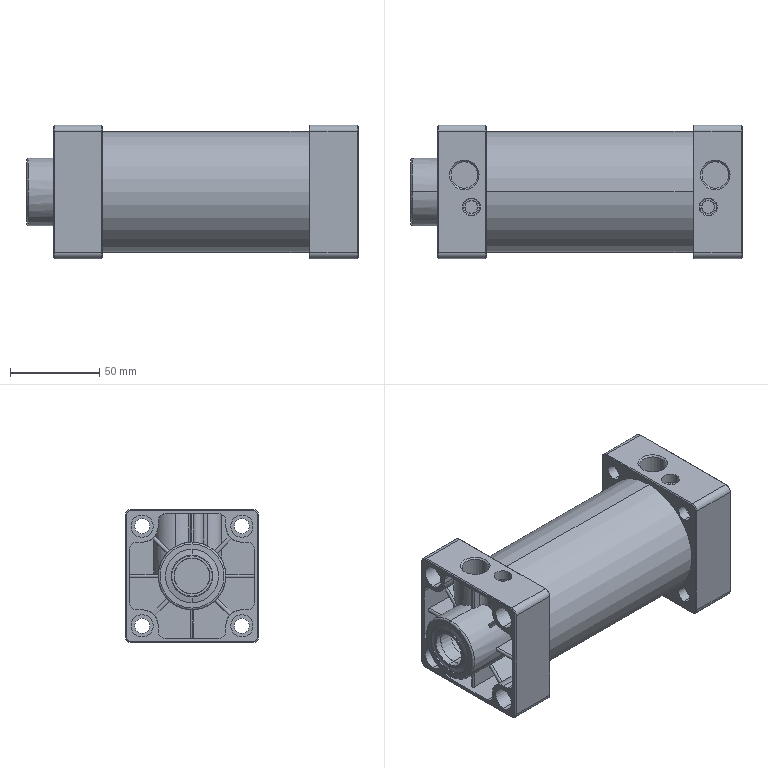Part | STEP file | 1 solid | 298 faces | box 186.5 x 75 x 75 mm | volume 216850 mm3 | cylinder 134 | plane 126 | cone 30 | torus 8 | commonest cylinder face diameters 8 x19 2.2 x18 8.5 x16 12.5 x16 7 x12 18 x8